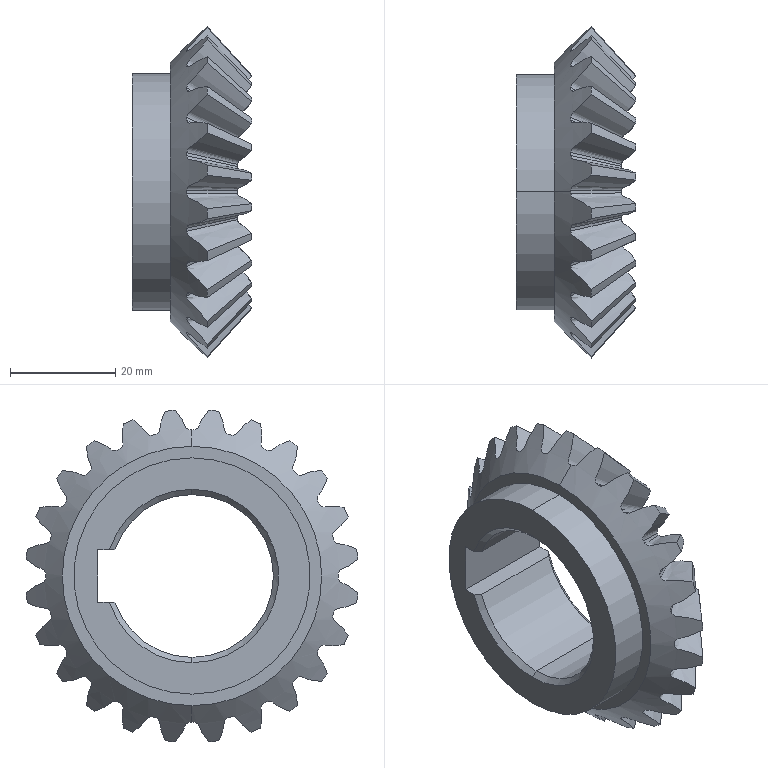Part | SolidWorks | features ICE 2, BlendCut 1, Chamfer 1, CirPattern 1, RefAxis 1, Revolution 1 | 1 solid | 117 faces | box 22.784 x 63.218 x 63.218 mm | volume 24670 mm3 | spline 72 | cone 34 | plane 6 | cylinder 5 | commonest cylinder face diameters 31 x3 45 x2